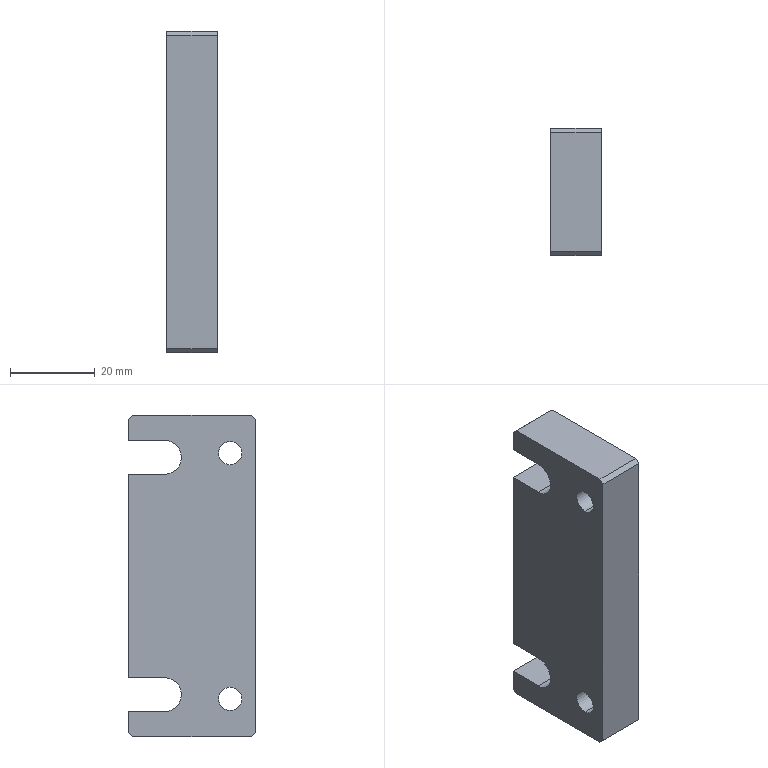Part | STEP file | support plate 27_SUS304 | 1 solid | 28 faces | box 12 x 30 x 76 mm | volume 23983 mm3 | plane 18 | cylinder 10 | commonest cylinder face diameters 5.5 x4 10 x4 8 x2